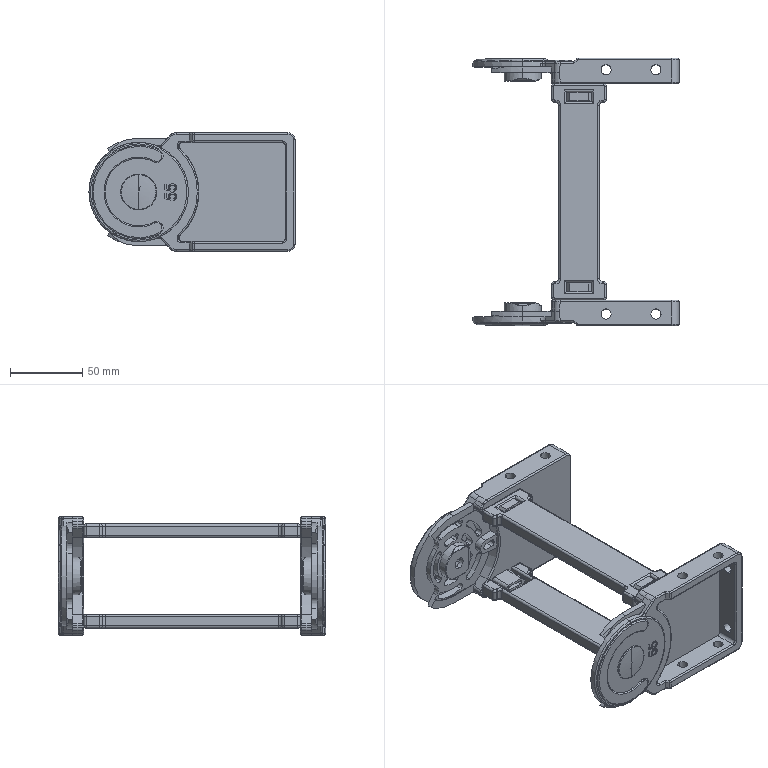Part | SolidWorks | features MirrorCompFeat 1, ReferencePattern 1 | 4 solids | 978 faces | box 142.639 x 185 x 82 mm | volume 215082 mm3 | plane 332 | cylinder 274 | cone 194 | torus 120 | spline 46 | sphere 12 | commonest cylinder face diameters 3 x80 2 x50 4 x28 7 x24 4.4 x12 10 x12